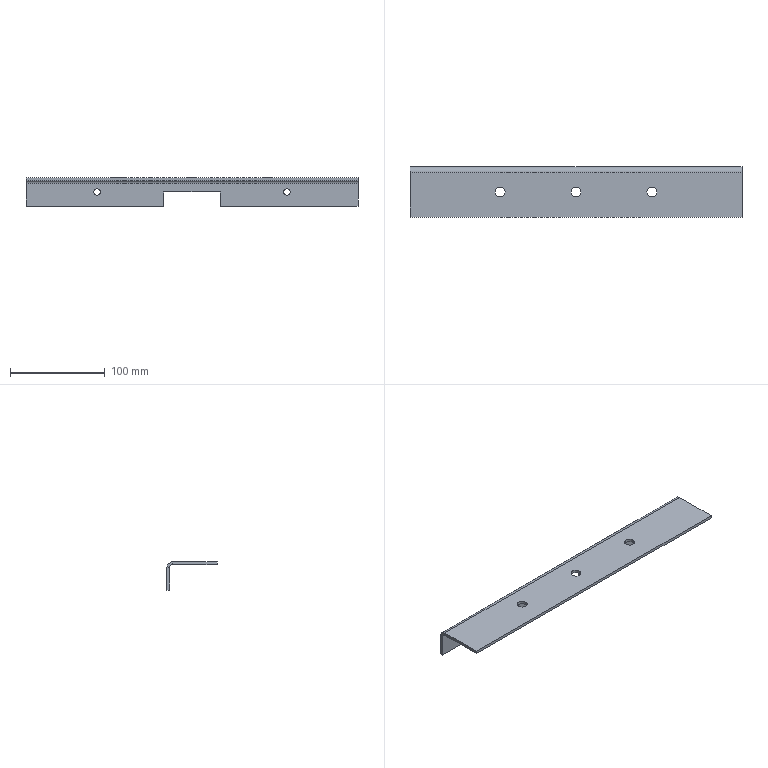Part | SolidWorks | features ICE 3, FlatPattern 1, SMBaseFlange 1, SheetMetal 1 | 1 solid | 28 faces | box 350 x 53 x 30 mm | volume 78262 mm3 | plane 16 | cylinder 12 | commonest cylinder face diameters 10.5 x6 7 x4 6 x1 12 x1
STEP:
#1=CARTESIAN_POINT('',(-100.,-3.,-18.5));
#2=VERTEX_POINT('',#1);
#3=CARTESIAN_POINT('',(-100.,-3.,-11.5));
#4=VERTEX_POINT('',#3);
#5=CARTESIAN_POINT('',(-100.,-3.,-15.));
#6=DIRECTION('',(0.,1.,0.));
#7=DIRECTION('',(0.,0.,-1.));
#8=AXIS2_PLACEMENT_3D('',#5,#6,#7);
#9=CIRCLE('',#8,3.5);
#10=EDGE_CURVE('',#2,#4,#9,.T.);
#11=ORIENTED_EDGE('',*,*,#10,.F.);
#12=CARTESIAN_POINT('',(-100.,0.,-18.5));
#13=VERTEX_POINT('',#12);
#14=CARTESIAN_POINT('',(-100.,-53.001,-18.5));
#15=DIRECTION('',(0.,1.,0.));
#16=VECTOR('',#15,1000.);
#17=LINE('',#14,#16);
#18=EDGE_CURVE('',#2,#13,#17,.T.);
#19=ORIENTED_EDGE('',*,*,#18,.T.);
#20=CARTESIAN_POINT('',(-100.,0.,-11.5));
#21=VERTEX_POINT('',#20);
#22=CARTESIAN_POINT('',(-100.,0.,-15.));
#23=DIRECTION('',(0.,1.,0.));
#24=DIRECTION('',(0.,0.,1.));
#25=AXIS2_PLACEMENT_3D('',#22,#23,#24);
#26=CIRCLE('',#25,3.5);
#27=EDGE_CURVE('',#13,#21,#26,.T.);
#28=ORIENTED_EDGE('',*,*,#27,.T.);
#29=CARTESIAN_POINT('',(-100.,-53.001,-11.5));
#30=DIRECTION('',(0.,1.,0.));
#31=VECTOR('',#30,1000.);
#32=LINE('',#29,#31);
#33=EDGE_CURVE('',#4,#21,#32,.T.);
#34=ORIENTED_EDGE('',*,*,#33,.F.);
#35=EDGE_LOOP('',(#11,#19,#28,#34));
#36=FACE_OUTER_BOUND('',#35,.T.);
#37=CARTESIAN_POINT('',(-100.,-53.001,-15.));
#38=DIRECTION('',(0.,1.,0.));
#39=DIRECTION('',(0.,0.,1.));
#40=AXIS2_PLACEMENT_3D('',#37,#38,#39);
#41=CYLINDRICAL_SURFACE('',#40,3.5);
#42=ADVANCED_FACE('',(#36),#41,.F.);
#43=CARTESIAN_POINT('',(100.,-3.,-18.5));
#44=VERTEX_POINT('',#43);
#45=CARTESIAN_POINT('',(100.,-3.,-11.5));
#46=VERTEX_POINT('',#45);
#47=CARTESIAN_POINT('',(100.,-3.,-15.));
#48=DIRECTION('',(0.,1.,0.));
#49=DIRECTION('',(0.,0.,-1.));
#50=AXIS2_PLACEMENT_3D('',#47,#48,#49);
#51=CIRCLE('',#50,3.5);
#52=EDGE_CURVE('',#44,#46,#51,.T.);
#53=ORIENTED_EDGE('',*,*,#52,.F.);
#54=CARTESIAN_POINT('',(100.,0.,-18.5));
#55=VERTEX_POINT('',#54);
#56=CARTESIAN_POINT('',(100.,-53.001,-18.5));
#57=DIRECTION('',(0.,1.,0.));
#58=VECTOR('',#57,1000.);
#59=LINE('',#56,#58);
#60=EDGE_CURVE('',#44,#55,#59,.T.);
#61=ORIENTED_EDGE('',*,*,#60,.T.);
#62=CARTESIAN_POINT('',(100.,0.,-11.5));
#63=VERTEX_POINT('',#62);
#64=CARTESIAN_POINT('',(100.,0.,-15.));
#65=DIRECTION('',(0.,1.,0.));
#66=DIRECTION('',(0.,0.,-1.));
#67=AXIS2_PLACEMENT_3D('',#64,#65,#66);
#68=CIRCLE('',#67,3.5);
#69=EDGE_CURVE('',#55,#63,#68,.T.);
#70=ORIENTED_EDGE('',*,*,#69,.T.);
#71=CARTESIAN_POINT('',(100.,-53.001,-11.5));
#72=DIRECTION('',(0.,1.,0.));
#73=VECTOR('',#72,1000.);
#74=LINE('',#71,#73);
#75=EDGE_CURVE('',#46,#63,#74,.T.);
#76=ORIENTED_EDGE('',*,*,#75,.F.);
#77=EDGE_LOOP('',(#53,#61,#70,#76));
#78=FACE_OUTER_BOUND('',#77,.T.);
#79=CARTESIAN_POINT('',(100.,-53.001,-15.));
#80=DIRECTION('',(0.,1.,0.));
#81=DIRECTION('',(0.,0.,1.));
#82=AXIS2_PLACEMENT_3D('',#79,#80,#81);
#83=CYLINDRICAL_SURFACE('',#82,3.5);
#84=ADVANCED_FACE('',(#78),#83,.F.);
#85=CARTESIAN_POINT('',(-74.75,-26.5,-3.));
#86=VERTEX_POINT('',#85);
#87=CARTESIAN_POINT('',(-85.25,-26.5,-3.));
#88=VERTEX_POINT('',#87);
#89=CARTESIAN_POINT('',(-80.,-26.5,-3.));
#90=DIRECTION('',(0.,0.,-1.));
#91=DIRECTION('',(-1.,0.,0.));
#92=AXIS2_PLACEMENT_3D('',#89,#90,#91);
#93=CIRCLE('',#92,5.25);
#94=EDGE_CURVE('',#86,#88,#93,.T.);
#95=ORIENTED_EDGE('',*,*,#94,.T.);
#96=CARTESIAN_POINT('',(-85.25,-26.5,0.));
#97=VERTEX_POINT('',#96);
#98=CARTESIAN_POINT('',(-85.25,-26.5,-30.));
#99=DIRECTION('',(0.,0.,1.));
#100=VECTOR('',#99,1000.);
#101=LINE('',#98,#100);
#102=EDGE_CURVE('',#88,#97,#101,.T.);
#103=ORIENTED_EDGE('',*,*,#102,.T.);
#104=CARTESIAN_POINT('',(-74.75,-26.5,0.));
#105=VERTEX_POINT('',#104);
#106=CARTESIAN_POINT('',(-80.,-26.5,0.));
#107=DIRECTION('',(0.,0.,1.));
#108=DIRECTION('',(1.,0.,0.));
#109=AXIS2_PLACEMENT_3D('',#106,#107,#108);
#110=CIRCLE('',#109,5.25);
#111=EDGE_CURVE('',#97,#105,#110,.T.);
#112=ORIENTED_EDGE('',*,*,#111,.T.);
#113=CARTESIAN_POINT('',(-74.75,-26.5,-30.));
#114=DIRECTION('',(0.,0.,1.));
#115=VECTOR('',#114,1000.);
#116=LINE('',#113,#115);
#117=EDGE_CURVE('',#86,#105,#116,.T.);
#118=ORIENTED_EDGE('',*,*,#117,.F.);
#119=EDGE_LOOP('',(#95,#103,#112,#118));
#120=FACE_OUTER_BOUND('',#119,.T.);
#121=CARTESIAN_POINT('',(-80.,-26.5,-30.));
#122=DIRECTION('',(0.,0.,1.));
#123=DIRECTION('',(1.,0.,0.));
#124=AXIS2_PLACEMENT_3D('',#121,#122,#123);
#125=CYLINDRICAL_SURFACE('',#124,5.25);
#126=ADVANCED_FACE('',(#120),#125,.F.);
#127=CARTESIAN_POINT('',(85.25,-26.5,-3.));
#128=VERTEX_POINT('',#127);
#129=CARTESIAN_POINT('',(74.75,-26.5,-3.));
#130=VERTEX_POINT('',#129);
#131=CARTESIAN_POINT('',(80.,-26.5,-3.));
#132=DIRECTION('',(0.,0.,-1.));
#133=DIRECTION('',(-1.,0.,0.));
#134=AXIS2_PLACEMENT_3D('',#131,#132,#133);
#135=CIRCLE('',#134,5.25);
#136=EDGE_CURVE('',#128,#130,#135,.T.);
#137=ORIENTED_EDGE('',*,*,#136,.T.);
#138=CARTESIAN_POINT('',(74.75,-26.5,0.));
#139=VERTEX_POINT('',#138);
#140=CARTESIAN_POINT('',(74.75,-26.5,-30.));
#141=DIRECTION('',(0.,0.,1.));
#142=VECTOR('',#141,1000.);
#143=LINE('',#140,#142);
#144=EDGE_CURVE('',#130,#139,#143,.T.);
#145=ORIENTED_EDGE('',*,*,#144,.T.);
#146=CARTESIAN_POINT('',(85.25,-26.5,0.));
#147=VERTEX_POINT('',#146);
#148=CARTESIAN_POINT('',(80.,-26.5,0.));
#149=DIRECTION('',(0.,0.,1.));
#150=DIRECTION('',(1.,0.,0.));
#151=AXIS2_PLACEMENT_3D('',#148,#149,#150);
#152=CIRCLE('',#151,5.25);
#153=EDGE_CURVE('',#139,#147,#152,.T.);
#154=ORIENTED_EDGE('',*,*,#153,.T.);
#155=CARTESIAN_POINT('',(85.25,-26.5,-30.));
#156=DIRECTION('',(0.,0.,1.));
#157=VECTOR('',#156,1000.);
#158=LINE('',#155,#157);
#159=EDGE_CURVE('',#128,#147,#158,.T.);
#160=ORIENTED_EDGE('',*,*,#159,.F.);
#161=EDGE_LOOP('',(#137,#145,#154,#160));
#162=FACE_OUTER_BOUND('',#161,.T.);
#163=CARTESIAN_POINT('',(80.,-26.5,-30.));
#164=DIRECTION('',(0.,0.,1.));
#165=DIRECTION('',(1.,0.,0.));
#166=AXIS2_PLACEMENT_3D('',#163,#164,#165);
#167=CYLINDRICAL_SURFACE('',#166,5.25);
#168=ADVANCED_FACE('',(#162),#167,.F.);
#169=CARTESIAN_POINT('',(5.25,-26.5,-3.));
#170=VERTEX_POINT('',#169);
#171=CARTESIAN_POINT('',(-5.25,-26.5,-3.));
#172=VERTEX_POINT('',#171);
#173=CARTESIAN_POINT('',(0.,-26.5,-3.));
#174=DIRECTION('',(0.,0.,-1.));
#175=DIRECTION('',(-1.,0.,0.));
#176=AXIS2_PLACEMENT_3D('',#173,#174,#175);
#177=CIRCLE('',#176,5.25);
#178=EDGE_CURVE('',#170,#172,#177,.T.);
#179=ORIENTED_EDGE('',*,*,#178,.T.);
#180=CARTESIAN_POINT('',(-5.25,-26.5,0.));
#181=VERTEX_POINT('',#180);
#182=CARTESIAN_POINT('',(-5.25,-26.5,-30.));
#183=DIRECTION('',(0.,0.,1.));
#184=VECTOR('',#183,1000.);
#185=LINE('',#182,#184);
#186=EDGE_CURVE('',#172,#181,#185,.T.);
#187=ORIENTED_EDGE('',*,*,#186,.T.);
#188=CARTESIAN_POINT('',(5.25,-26.5,0.));
#189=VERTEX_POINT('',#188);
#190=CARTESIAN_POINT('',(0.,-26.5,0.));
#191=DIRECTION('',(0.,0.,1.));
#192=DIRECTION('',(1.,0.,0.));
#193=AXIS2_PLACEMENT_3D('',#190,#191,#192);
#194=CIRCLE('',#193,5.25);
#195=EDGE_CURVE('',#181,#189,#194,.T.);
#196=ORIENTED_EDGE('',*,*,#195,.T.);
#197=CARTESIAN_POINT('',(5.25,-26.5,-30.));
#198=DIRECTION('',(0.,0.,1.));
#199=VECTOR('',#198,1000.);
#200=LINE('',#197,#199);
#201=EDGE_CURVE('',#170,#189,#200,.T.);
#202=ORIENTED_EDGE('',*,*,#201,.F.);
#203=EDGE_LOOP('',(#179,#187,#196,#202));
#204=FACE_OUTER_BOUND('',#203,.T.);
#205=CARTESIAN_POINT('',(0.,-26.5,-30.));
#206=DIRECTION('',(0.,0.,1.));
#207=DIRECTION('',(1.,0.,0.));
#208=AXIS2_PLACEMENT_3D('',#205,#206,#207);
#209=CYLINDRICAL_SURFACE('',#208,5.25);
#210=ADVANCED_FACE('',(#204),#209,.F.);
#211=CARTESIAN_POINT('',(30.,0.,-30.));
#212=VERTEX_POINT('',#211);
#213=CARTESIAN_POINT('',(30.,-3.,-30.));
#214=VERTEX_POINT('',#213);
#215=CARTESIAN_POINT('',(30.,0.,-30.));
#216=DIRECTION('',(0.,-1.,0.));
#217=VECTOR('',#216,1000.);
#218=LINE('',#215,#217);
#219=EDGE_CURVE('',#212,#214,#218,.T.);
#220=ORIENTED_EDGE('',*,*,#219,.F.);
#221=CARTESIAN_POINT('',(175.,0.,-30.));
#222=VERTEX_POINT('',#221);
#223=CARTESIAN_POINT('',(175.,0.,-30.));
#224=DIRECTION('',(-1.,0.,0.));
#225=VECTOR('',#224,1000.);
#226=LINE('',#223,#225);
#227=EDGE_CURVE('',#222,#212,#226,.T.);
#228=ORIENTED_EDGE('',*,*,#227,.F.);
#229=CARTESIAN_POINT('',(175.,-3.,-30.));
#230=VERTEX_POINT('',#229);
#231=CARTESIAN_POINT('',(175.,0.,-30.));
#232=DIRECTION('',(0.,-1.,0.));
#233=VECTOR('',#232,1000.);
#234=LINE('',#231,#233);
#235=EDGE_CURVE('',#222,#230,#234,.T.);
#236=ORIENTED_EDGE('',*,*,#235,.T.);
#237=CARTESIAN_POINT('',(175.,-3.,-30.));
#238=DIRECTION('',(-1.,0.,0.));
#239=VECTOR('',#238,1000.);
#240=LINE('',#237,#239);
#241=EDGE_CURVE('',#230,#214,#240,.T.);
#242=ORIENTED_EDGE('',*,*,#241,.T.);
#243=EDGE_LOOP('',(#220,#228,#236,#242));
#244=FACE_OUTER_BOUND('',#243,.T.);
#245=CARTESIAN_POINT('',(175.,0.,-30.));
#246=DIRECTION('',(0.,0.,-1.));
#247=DIRECTION('',(-1.,0.,0.));
#248=AXIS2_PLACEMENT_3D('',#245,#246,#247);
#249=PLANE('',#248);
#250=ADVANCED_FACE('',(#244),#249,.T.);
#251=CARTESIAN_POINT('',(175.,0.,-6.));
#252=VERTEX_POINT('',#251);
#253=CARTESIAN_POINT('',(175.,-3.,-6.));
#254=VERTEX_POINT('',#253);
#255=CARTESIAN_POINT('',(175.,0.,-6.));
#256=DIRECTION('',(0.,-1.,0.));
#257=VECTOR('',#256,1000.);
#258=LINE('',#255,#257);
#259=EDGE_CURVE('',#252,#254,#258,.T.);
#260=ORIENTED_EDGE('',*,*,#259,.F.);
#261=CARTESIAN_POINT('',(175.,-6.,0.));
#262=VERTEX_POINT('',#261);
#263=CARTESIAN_POINT('',(175.,-6.,-6.));
#264=DIRECTION('',(1.,0.,0.));
#265=DIRECTION('',(0.,0.,1.));
#266=AXIS2_PLACEMENT_3D('',#263,#264,#265);
#267=CIRCLE('',#266,6.);
#268=EDGE_CURVE('',#252,#262,#267,.T.);
#269=ORIENTED_EDGE('',*,*,#268,.T.);
#270=CARTESIAN_POINT('',(175.,-6.,-3.));
#271=VERTEX_POINT('',#270);
#272=CARTESIAN_POINT('',(175.,-6.,-3.));
#273=DIRECTION('',(0.,0.,1.));
#274=VECTOR('',#273,1000.);
#275=LINE('',#272,#274);
#276=EDGE_CURVE('',#271,#262,#275,.T.);
#277=ORIENTED_EDGE('',*,*,#276,.F.);
#278=CARTESIAN_POINT('',(175.,-6.,-6.));
#279=DIRECTION('',(1.,0.,0.));
#280=DIRECTION('',(0.,0.,-1.));
#281=AXIS2_PLACEMENT_3D('',#278,#279,#280);
#282=CIRCLE('',#281,3.);
#283=EDGE_CURVE('',#254,#271,#282,.T.);
#284=ORIENTED_EDGE('',*,*,#283,.F.);
#285=EDGE_LOOP('',(#260,#269,#277,#284));
#286=FACE_OUTER_BOUND('',#285,.T.);
#287=CARTESIAN_POINT('',(175.,0.,-6.));
#288=DIRECTION('',(1.,0.,0.));
#289=DIRECTION('',(0.,0.,-1.));
#290=AXIS2_PLACEMENT_3D('',#287,#288,#289);
#291=PLANE('',#290);
#292=ADVANCED_FACE('',(#286),#291,.T.);
#293=CARTESIAN_POINT('',(175.,0.,-30.));
#294=DIRECTION('',(0.,0.,1.));
#295=VECTOR('',#294,1000.);
#296=LINE('',#293,#295);
#297=EDGE_CURVE('',#222,#252,#296,.T.);
#298=ORIENTED_EDGE('',*,*,#297,.T.);
#299=ORIENTED_EDGE('',*,*,#259,.T.);
#300=CARTESIAN_POINT('',(175.,-3.,-30.));
#301=DIRECTION('',(0.,0.,1.));
#302=VECTOR('',#301,1000.);
#303=LINE('',#300,#302);
#304=EDGE_CURVE('',#230,#254,#303,.T.);
#305=ORIENTED_EDGE('',*,*,#304,.F.);
#306=ORIENTED_EDGE('',*,*,#235,.F.);
#307=EDGE_LOOP('',(#298,#299,#305,#306));
#308=FACE_OUTER_BOUND('',#307,.T.);
#309=CARTESIAN_POINT('',(175.,-6.,-3.));
#310=DIRECTION('',(1.,0.,0.));
#311=DIRECTION('',(0.,0.,-1.));
#312=AXIS2_PLACEMENT_3D('',#309,#310,#311);
#313=PLANE('',#312);
#314=ADVANCED_FACE('',(#308),#313,.T.);
#315=CARTESIAN_POINT('',(-175.,-6.,0.));
#316=VERTEX_POINT('',#315);
#317=CARTESIAN_POINT('',(-175.,-6.,-3.));
#318=VERTEX_POINT('',#317);
#319=CARTESIAN_POINT('',(-175.,-6.,0.));
#320=DIRECTION('',(0.,0.,-1.));
#321=VECTOR('',#320,1000.);
#322=LINE('',#319,#321);
#323=EDGE_CURVE('',#316,#318,#322,.T.);
#324=ORIENTED_EDGE('',*,*,#323,.F.);
#325=CARTESIAN_POINT('',(-175.,0.,-6.));
#326=VERTEX_POINT('',#325);
#327=CARTESIAN_POINT('',(-175.,-6.,-6.));
#328=DIRECTION('',(1.,0.,0.));
#329=DIRECTION('',(0.,0.,1.));
#330=AXIS2_PLACEMENT_3D('',#327,#328,#329);
#331=CIRCLE('',#330,6.);
#332=EDGE_CURVE('',#326,#316,#331,.T.);
#333=ORIENTED_EDGE('',*,*,#332,.F.);
#334=CARTESIAN_POINT('',(-175.,-3.,-6.));
#335=VERTEX_POINT('',#334);
#336=CARTESIAN_POINT('',(-175.,-3.,-6.));
#337=DIRECTION('',(0.,1.,0.));
#338=VECTOR('',#337,1000.);
#339=LINE('',#336,#338);
#340=EDGE_CURVE('',#335,#326,#339,.T.);
#341=ORIENTED_EDGE('',*,*,#340,.F.);
#342=CARTESIAN_POINT('',(-175.,-6.,-6.));
#343=DIRECTION('',(1.,0.,0.));
#344=DIRECTION('',(0.,0.,-1.));
#345=AXIS2_PLACEMENT_3D('',#342,#343,#344);
#346=CIRCLE('',#345,3.);
#347=EDGE_CURVE('',#335,#318,#346,.T.);
#348=ORIENTED_EDGE('',*,*,#347,.T.);
#349=EDGE_LOOP('',(#324,#333,#341,#348));
#350=FACE_OUTER_BOUND('',#349,.T.);
#351=CARTESIAN_POINT('',(-175.,-6.,0.));
#352=DIRECTION('',(-1.,0.,0.));
#353=DIRECTION('',(0.,0.,1.));
#354=AXIS2_PLACEMENT_3D('',#351,#352,#353);
#355=PLANE('',#354);
#356=ADVANCED_FACE('',(#350),#355,.T.);
#357=CARTESIAN_POINT('',(-175.,-53.,0.));
#358=VERTEX_POINT('',#357);
#359=CARTESIAN_POINT('',(-175.,0.,0.));
#360=DIRECTION('',(0.,-1.,0.));
#361=VECTOR('',#360,1000.);
#362=LINE('',#359,#361);
#363=EDGE_CURVE('',#316,#358,#362,.T.);
#364=ORIENTED_EDGE('',*,*,#363,.F.);
#365=ORIENTED_EDGE('',*,*,#323,.T.);
#366=CARTESIAN_POINT('',(-175.,-53.,-3.));
#367=VERTEX_POINT('',#366);
#368=CARTESIAN_POINT('',(-175.,0.,-3.));
#369=DIRECTION('',(0.,-1.,0.));
#370=VECTOR('',#369,1000.);
#371=LINE('',#368,#370);
#372=EDGE_CURVE('',#318,#367,#371,.T.);
#373=ORIENTED_EDGE('',*,*,#372,.T.);
#374=CARTESIAN_POINT('',(-175.,-53.,-3.));
#375=DIRECTION('',(0.,0.,1.));
#376=VECTOR('',#375,1000.);
#377=LINE('',#374,#376);
#378=EDGE_CURVE('',#367,#358,#377,.T.);
#379=ORIENTED_EDGE('',*,*,#378,.T.);
#380=EDGE_LOOP('',(#364,#365,#373,#379));
#381=FACE_OUTER_BOUND('',#380,.T.);
#382=CARTESIAN_POINT('',(-175.,-3.,-6.));
#383=DIRECTION('',(-1.,0.,0.));
#384=DIRECTION('',(0.,0.,1.));
#385=AXIS2_PLACEMENT_3D('',#382,#383,#384);
#386=PLANE('',#385);
#387=ADVANCED_FACE('',(#381),#386,.T.);
#388=CARTESIAN_POINT('',(-80.,-26.5,0.));
#389=DIRECTION('',(0.,0.,1.));
#390=DIRECTION('',(1.,0.,0.));
#391=AXIS2_PLACEMENT_3D('',#388,#389,#390);
#392=CIRCLE('',#391,5.25);
#393=EDGE_CURVE('',#105,#97,#392,.T.);
#394=ORIENTED_EDGE('',*,*,#393,.F.);
#395=ORIENTED_EDGE('',*,*,#111,.F.);
#396=EDGE_LOOP('',(#394,#395));
#397=FACE_BOUND('',#396,.T.);
#398=CARTESIAN_POINT('',(80.,-26.5,0.));
#399=DIRECTION('',(0.,0.,1.));
#400=DIRECTION('',(1.,0.,0.));
#401=AXIS2_PLACEMENT_3D('',#398,#399,#400);
#402=CIRCLE('',#401,5.25);
#403=EDGE_CURVE('',#147,#139,#402,.T.);
#404=ORIENTED_EDGE('',*,*,#403,.F.);
#405=ORIENTED_EDGE('',*,*,#153,.F.);
#406=EDGE_LOOP('',(#404,#405));
#407=FACE_BOUND('',#406,.T.);
#408=CARTESIAN_POINT('',(0.,-26.5,0.));
#409=DIRECTION('',(0.,0.,1.));
#410=DIRECTION('',(1.,0.,0.));
#411=AXIS2_PLACEMENT_3D('',#408,#409,#410);
#412=CIRCLE('',#411,5.25);
#413=EDGE_CURVE('',#189,#181,#412,.T.);
#414=ORIENTED_EDGE('',*,*,#413,.F.);
#415=ORIENTED_EDGE('',*,*,#195,.F.);
#416=EDGE_LOOP('',(#414,#415));
#417=FACE_BOUND('',#416,.T.);
#418=ORIENTED_EDGE('',*,*,#363,.T.);
#419=CARTESIAN_POINT('',(175.,-53.,0.));
#420=VERTEX_POINT('',#419);
#421=CARTESIAN_POINT('',(175.,-53.,0.));
#422=DIRECTION('',(-1.,0.,0.));
#423=VECTOR('',#422,1000.);
#424=LINE('',#421,#423);
#425=EDGE_CURVE('',#420,#358,#424,.T.);
#426=ORIENTED_EDGE('',*,*,#425,.F.);
#427=CARTESIAN_POINT('',(175.,0.,0.));
#428=DIRECTION('',(0.,-1.,0.));
#429=VECTOR('',#428,1000.);
#430=LINE('',#427,#429);
#431=EDGE_CURVE('',#262,#420,#430,.T.);
#432=ORIENTED_EDGE('',*,*,#431,.F.);
#433=CARTESIAN_POINT('',(175.,-6.,0.));
#434=DIRECTION('',(-1.,0.,0.));
#435=VECTOR('',#434,1000.);
#436=LINE('',#433,#435);
#437=EDGE_CURVE('',#262,#316,#436,.T.);
#438=ORIENTED_EDGE('',*,*,#437,.T.);
#439=EDGE_LOOP('',(#418,#426,#432,#438));
#440=FACE_OUTER_BOUND('',#439,.T.);
#441=CARTESIAN_POINT('',(175.,0.,0.));
#442=DIRECTION('',(0.,0.,-1.));
#443=DIRECTION('',(-1.,0.,0.));
#444=AXIS2_PLACEMENT_3D('',#441,#442,#443);
#445=PLANE('',#444);
#446=ADVANCED_FACE('',(#397,#407,#417,#440),#445,.F.);
#447=ORIENTED_EDGE('',*,*,#378,.F.);
#448=CARTESIAN_POINT('',(175.,-53.,-3.));
#449=VERTEX_POINT('',#448);
#450=CARTESIAN_POINT('',(175.,-53.,-3.));
#451=DIRECTION('',(-1.,0.,0.));
#452=VECTOR('',#451,1000.);
#453=LINE('',#450,#452);
#454=EDGE_CURVE('',#449,#367,#453,.T.);
#455=ORIENTED_EDGE('',*,*,#454,.F.);
#456=CARTESIAN_POINT('',(175.,-53.,-3.));
#457=DIRECTION('',(0.,0.,1.));
#458=VECTOR('',#457,1000.);
#459=LINE('',#456,#458);
#460=EDGE_CURVE('',#449,#420,#459,.T.);
#461=ORIENTED_EDGE('',*,*,#460,.T.);
#462=ORIENTED_EDGE('',*,*,#425,.T.);
#463=EDGE_LOOP('',(#447,#455,#461,#462));
#464=FACE_OUTER_BOUND('',#463,.T.);
#465=CARTESIAN_POINT('',(175.,-53.,-3.));
#466=DIRECTION('',(0.,-1.,0.));
#467=DIRECTION('',(0.,0.,-1.));
#468=AXIS2_PLACEMENT_3D('',#465,#466,#467);
#469=PLANE('',#468);
#470=ADVANCED_FACE('',(#464),#469,.T.);
#471=ORIENTED_EDGE('',*,*,#94,.F.);
#472=CARTESIAN_POINT('',(-80.,-26.5,-3.));
#473=DIRECTION('',(0.,0.,-1.));
#474=DIRECTION('',(-1.,0.,0.));
#475=AXIS2_PLACEMENT_3D('',#472,#473,#474);
#476=CIRCLE('',#475,5.25);
#477=EDGE_CURVE('',#88,#86,#476,.T.);
#478=ORIENTED_EDGE('',*,*,#477,.F.);
#479=EDGE_LOOP('',(#471,#478));
#480=FACE_BOUND('',#479,.T.);
#481=ORIENTED_EDGE('',*,*,#136,.F.);
#482=CARTESIAN_POINT('',(80.,-26.5,-3.));
#483=DIRECTION('',(0.,0.,-1.));
#484=DIRECTION('',(-1.,0.,0.));
#485=AXIS2_PLACEMENT_3D('',#482,#483,#484);
#486=CIRCLE('',#485,5.25);
#487=EDGE_CURVE('',#130,#128,#486,.T.);
#488=ORIENTED_EDGE('',*,*,#487,.F.);
#489=EDGE_LOOP('',(#481,#488));
#490=FACE_BOUND('',#489,.T.);
#491=ORIENTED_EDGE('',*,*,#178,.F.);
#492=CARTESIAN_POINT('',(0.,-26.5,-3.));
#493=DIRECTION('',(0.,0.,-1.));
#494=DIRECTION('',(-1.,0.,0.));
#495=AXIS2_PLACEMENT_3D('',#492,#493,#494);
#496=CIRCLE('',#495,5.25);
#497=EDGE_CURVE('',#172,#170,#496,.T.);
#498=ORIENTED_EDGE('',*,*,#497,.F.);
#499=EDGE_LOOP('',(#491,#498));
#500=FACE_BOUND('',#499,.T.);
#501=ORIENTED_EDGE('',*,*,#372,.F.);
#502=CARTESIAN_POINT('',(175.,-6.,-3.));
#503=DIRECTION('',(-1.,0.,0.));
#504=VECTOR('',#503,1000.);
#505=LINE('',#502,#504);
#506=EDGE_CURVE('',#271,#318,#505,.T.);
#507=ORIENTED_EDGE('',*,*,#506,.F.);
#508=CARTESIAN_POINT('',(175.,0.,-3.));
#509=DIRECTION('',(0.,-1.,0.));
#510=VECTOR('',#509,1000.);
#511=LINE('',#508,#510);
#512=EDGE_CURVE('',#271,#449,#511,.T.);
#513=ORIENTED_EDGE('',*,*,#512,.T.);
#514=ORIENTED_EDGE('',*,*,#454,.T.);
#515=EDGE_LOOP('',(#501,#507,#513,#514));
#516=FACE_OUTER_BOUND('',#515,.T.);
#517=CARTESIAN_POINT('',(175.,0.,-3.));
#518=DIRECTION('',(0.,0.,-1.));
#519=DIRECTION('',(-1.,0.,0.));
#520=AXIS2_PLACEMENT_3D('',#517,#518,#519);
#521=PLANE('',#520);
#522=ADVANCED_FACE('',(#480,#490,#500,#516),#521,.T.);
#523=ORIENTED_EDGE('',*,*,#347,.F.);
#524=CARTESIAN_POINT('',(175.,-3.,-6.));
#525=DIRECTION('',(-1.,0.,0.));
#526=VECTOR('',#525,1000.);
#527=LINE('',#524,#526);
#528=EDGE_CURVE('',#254,#335,#527,.T.);
#529=ORIENTED_EDGE('',*,*,#528,.F.);
#530=ORIENTED_EDGE('',*,*,#283,.T.);
#531=ORIENTED_EDGE('',*,*,#506,.T.);
#532=EDGE_LOOP('',(#523,#529,#530,#531));
#533=FACE_OUTER_BOUND('',#532,.T.);
#534=CARTESIAN_POINT('',(175.,-6.,-6.));
#535=DIRECTION('',(-1.,0.,0.));
#536=DIRECTION('',(0.,0.,1.));
#537=AXIS2_PLACEMENT_3D('',#534,#535,#536);
#538=CYLINDRICAL_SURFACE('',#537,3.);
#539=ADVANCED_FACE('',(#533),#538,.F.);
#540=CARTESIAN_POINT('',(30.,-3.,-15.));
#541=VERTEX_POINT('',#540);
#542=CARTESIAN_POINT('',(30.,-3.,-30.));
#543=DIRECTION('',(0.,0.,1.));
#544=VECTOR('',#543,1000.);
#545=LINE('',#542,#544);
#546=EDGE_CURVE('',#214,#541,#545,.T.);
#547=ORIENTED_EDGE('',*,*,#546,.F.);
#548=ORIENTED_EDGE('',*,*,#241,.F.);
#549=ORIENTED_EDGE('',*,*,#304,.T.);
#550=ORIENTED_EDGE('',*,*,#528,.T.);
#551=CARTESIAN_POINT('',(-175.,-3.,-30.));
#552=VERTEX_POINT('',#551);
#553=CARTESIAN_POINT('',(-175.,-3.,-30.));
#554=DIRECTION('',(0.,0.,1.));
#555=VECTOR('',#554,1000.);
#556=LINE('',#553,#555);
#557=EDGE_CURVE('',#552,#335,#556,.T.);
#558=ORIENTED_EDGE('',*,*,#557,.F.);
#559=CARTESIAN_POINT('',(-30.,-3.,-30.));
#560=VERTEX_POINT('',#559);
#561=CARTESIAN_POINT('',(175.,-3.,-30.));
#562=DIRECTION('',(-1.,0.,0.));
#563=VECTOR('',#562,1000.);
#564=LINE('',#561,#563);
#565=EDGE_CURVE('',#560,#552,#564,.T.);
#566=ORIENTED_EDGE('',*,*,#565,.F.);
#567=CARTESIAN_POINT('',(-30.,-3.,-15.));
#568=VERTEX_POINT('',#567);
#569=CARTESIAN_POINT('',(-30.,-3.,-30.));
#570=DIRECTION('',(0.,0.,-1.));
#571=VECTOR('',#570,1000.);
#572=LINE('',#569,#571);
#573=EDGE_CURVE('',#568,#560,#572,.T.);
#574=ORIENTED_EDGE('',*,*,#573,.F.);
#575=CARTESIAN_POINT('',(175.,-3.,-15.));
#576=DIRECTION('',(-1.,0.,0.));
#577=VECTOR('',#576,1000.);
#578=LINE('',#575,#577);
#579=EDGE_CURVE('',#541,#568,#578,.T.);
#580=ORIENTED_EDGE('',*,*,#579,.F.);
#581=EDGE_LOOP('',(#547,#548,#549,#550,#558,#566,#574,#580));
#582=FACE_OUTER_BOUND('',#581,.T.);
#583=CARTESIAN_POINT('',(-100.,-3.,-15.));
#584=DIRECTION('',(0.,1.,0.));
#585=DIRECTION('',(0.,0.,-1.));
#586=AXIS2_PLACEMENT_3D('',#583,#584,#585);
#587=CIRCLE('',#586,3.5);
#588=EDGE_CURVE('',#4,#2,#587,.T.);
#589=ORIENTED_EDGE('',*,*,#588,.T.);
#590=ORIENTED_EDGE('',*,*,#10,.T.);
#591=EDGE_LOOP('',(#589,#590));
#592=FACE_BOUND('',#591,.T.);
#593=CARTESIAN_POINT('',(100.,-3.,-15.));
#594=DIRECTION('',(0.,1.,0.));
#595=DIRECTION('',(0.,0.,-1.));
#596=AXIS2_PLACEMENT_3D('',#593,#594,#595);
#597=CIRCLE('',#596,3.5);
#598=EDGE_CURVE('',#46,#44,#597,.T.);
#599=ORIENTED_EDGE('',*,*,#598,.T.);
#600=ORIENTED_EDGE('',*,*,#52,.T.);
#601=EDGE_LOOP('',(#599,#600));
#602=FACE_BOUND('',#601,.T.);
#603=CARTESIAN_POINT('',(175.,-3.,-30.));
#604=DIRECTION('',(0.,-1.,0.));
#605=DIRECTION('',(0.,0.,-1.));
#606=AXIS2_PLACEMENT_3D('',#603,#604,#605);
#607=PLANE('',#606);
#608=ADVANCED_FACE('',(#582,#592,#602),#607,.T.);
#609=CARTESIAN_POINT('',(-30.,0.,-30.));
#610=VERTEX_POINT('',#609);
#611=CARTESIAN_POINT('',(-30.,0.,-30.));
#612=DIRECTION('',(0.,1.,0.));
#613=VECTOR('',#612,1000.);
#614=LINE('',#611,#613);
#615=EDGE_CURVE('',#560,#610,#614,.T.);
#616=ORIENTED_EDGE('',*,*,#615,.F.);
#617=ORIENTED_EDGE('',*,*,#565,.T.);
#618=CARTESIAN_POINT('',(-175.,0.,-30.));
#619=VERTEX_POINT('',#618);
#620=CARTESIAN_POINT('',(-175.,0.,-30.));
#621=DIRECTION('',(0.,-1.,0.));
#622=VECTOR('',#621,1000.);
#623=LINE('',#620,#622);
#624=EDGE_CURVE('',#619,#552,#623,.T.);
#625=ORIENTED_EDGE('',*,*,#624,.F.);
#626=CARTESIAN_POINT('',(175.,0.,-30.));
#627=DIRECTION('',(-1.,0.,0.));
#628=VECTOR('',#627,1000.);
#629=LINE('',#626,#628);
#630=EDGE_CURVE('',#610,#619,#629,.T.);
#631=ORIENTED_EDGE('',*,*,#630,.F.);
#632=EDGE_LOOP('',(#616,#617,#625,#631));
#633=FACE_OUTER_BOUND('',#632,.T.);
#634=CARTESIAN_POINT('',(175.,0.,-30.));
#635=DIRECTION('',(0.,0.,-1.));
#636=DIRECTION('',(-1.,0.,0.));
#637=AXIS2_PLACEMENT_3D('',#634,#635,#636);
#638=PLANE('',#637);
#639=ADVANCED_FACE('',(#633),#638,.T.);
#640=CARTESIAN_POINT('',(-100.,0.,-15.));
#641=DIRECTION('',(0.,1.,0.));
#642=DIRECTION('',(0.,0.,1.));
#643=AXIS2_PLACEMENT_3D('',#640,#641,#642);
#644=CIRCLE('',#643,3.5);
#645=EDGE_CURVE('',#21,#13,#644,.T.);
#646=ORIENTED_EDGE('',*,*,#645,.F.);
#647=ORIENTED_EDGE('',*,*,#27,.F.);
#648=EDGE_LOOP('',(#646,#647));
#649=FACE_BOUND('',#648,.T.);
#650=CARTESIAN_POINT('',(100.,0.,-15.));
#651=DIRECTION('',(0.,1.,0.));
#652=DIRECTION('',(0.,0.,-1.));
#653=AXIS2_PLACEMENT_3D('',#650,#651,#652);
#654=CIRCLE('',#653,3.5);
#655=EDGE_CURVE('',#63,#55,#654,.T.);
#656=ORIENTED_EDGE('',*,*,#655,.F.);
#657=ORIENTED_EDGE('',*,*,#69,.F.);
#658=EDGE_LOOP('',(#656,#657));
#659=FACE_BOUND('',#658,.T.);
#660=ORIENTED_EDGE('',*,*,#227,.T.);
#661=CARTESIAN_POINT('',(30.,0.,-15.));
#662=VERTEX_POINT('',#661);
#663=CARTESIAN_POINT('',(30.,0.,-15.));
#664=DIRECTION('',(0.,0.,-1.));
#665=VECTOR('',#664,1000.);
#666=LINE('',#663,#665);
#667=EDGE_CURVE('',#662,#212,#666,.T.);
#668=ORIENTED_EDGE('',*,*,#667,.F.);
#669=CARTESIAN_POINT('',(-30.,0.,-15.));
#670=VERTEX_POINT('',#669);
#671=CARTESIAN_POINT('',(-30.,0.,-15.));
#672=DIRECTION('',(1.,0.,0.));
#673=VECTOR('',#672,1000.);
#674=LINE('',#671,#673);
#675=EDGE_CURVE('',#670,#662,#674,.T.);
#676=ORIENTED_EDGE('',*,*,#675,.F.);
#677=CARTESIAN_POINT('',(-30.,0.,-30.));
#678=DIRECTION('',(0.,0.,-1.));
#679=VECTOR('',#678,1000.);
#680=LINE('',#677,#679);
#681=EDGE_CURVE('',#670,#610,#680,.T.);
#682=ORIENTED_EDGE('',*,*,#681,.T.);
#683=ORIENTED_EDGE('',*,*,#630,.T.);
#684=CARTESIAN_POINT('',(-175.,0.,-30.));
#685=DIRECTION('',(0.,0.,1.));
#686=VECTOR('',#685,1000.);
#687=LINE('',#684,#686);
#688=EDGE_CURVE('',#619,#326,#687,.T.);
#689=ORIENTED_EDGE('',*,*,#688,.T.);
#690=CARTESIAN_POINT('',(175.,0.,-6.));
#691=DIRECTION('',(-1.,0.,0.));
#692=VECTOR('',#691,1000.);
#693=LINE('',#690,#692);
#694=EDGE_CURVE('',#252,#326,#693,.T.);
#695=ORIENTED_EDGE('',*,*,#694,.F.);
#696=ORIENTED_EDGE('',*,*,#297,.F.);
#697=EDGE_LOOP('',(#660,#668,#676,#682,#683,#689,#695,#696));
#698=FACE_OUTER_BOUND('',#697,.T.);
#699=CARTESIAN_POINT('',(175.,0.,-30.));
#700=DIRECTION('',(0.,-1.,0.));
#701=DIRECTION('',(0.,0.,-1.));
#702=AXIS2_PLACEMENT_3D('',#699,#700,#701);
#703=PLANE('',#702);
#704=ADVANCED_FACE('',(#649,#659,#698),#703,.F.);
#705=ORIENTED_EDGE('',*,*,#332,.T.);
#706=ORIENTED_EDGE('',*,*,#437,.F.);
#707=ORIENTED_EDGE('',*,*,#268,.F.);
#708=ORIENTED_EDGE('',*,*,#694,.T.);
#709=EDGE_LOOP('',(#705,#706,#707,#708));
#710=FACE_OUTER_BOUND('',#709,.T.);
#711=CARTESIAN_POINT('',(175.,-6.,-6.));
#712=DIRECTION('',(-1.,0.,0.));
#713=DIRECTION('',(0.,0.,1.));
#714=AXIS2_PLACEMENT_3D('',#711,#712,#713);
#715=CYLINDRICAL_SURFACE('',#714,6.);
#716=ADVANCED_FACE('',(#710),#715,.T.);
#717=ORIENTED_EDGE('',*,*,#431,.T.);
#718=ORIENTED_EDGE('',*,*,#460,.F.);
#719=ORIENTED_EDGE('',*,*,#512,.F.);
#720=ORIENTED_EDGE('',*,*,#276,.T.);
#721=EDGE_LOOP('',(#717,#718,#719,#720));
#722=FACE_OUTER_BOUND('',#721,.T.);
#723=CARTESIAN_POINT('',(175.,-6.,-6.));
#724=DIRECTION('',(1.,0.,0.));
#725=DIRECTION('',(0.,0.,-1.));
#726=AXIS2_PLACEMENT_3D('',#723,#724,#725);
#727=PLANE('',#726);
#728=ADVANCED_FACE('',(#722),#727,.T.);
#729=ORIENTED_EDGE('',*,*,#557,.T.);
#730=ORIENTED_EDGE('',*,*,#340,.T.);
#731=ORIENTED_EDGE('',*,*,#688,.F.);
#732=ORIENTED_EDGE('',*,*,#624,.T.);
#733=EDGE_LOOP('',(#729,#730,#731,#732));
#734=FACE_OUTER_BOUND('',#733,.T.);
#735=CARTESIAN_POINT('',(-175.,-6.,-6.));
#736=DIRECTION('',(1.,0.,0.));
#737=DIRECTION('',(0.,0.,-1.));
#738=AXIS2_PLACEMENT_3D('',#735,#736,#737);
#739=PLANE('',#738);
#740=ADVANCED_FACE('',(#734),#739,.F.);
#741=ORIENTED_EDGE('',*,*,#186,.F.);
#742=ORIENTED_EDGE('',*,*,#497,.T.);
#743=ORIENTED_EDGE('',*,*,#201,.T.);
#744=ORIENTED_EDGE('',*,*,#413,.T.);
#745=EDGE_LOOP('',(#741,#742,#743,#744));
#746=FACE_OUTER_BOUND('',#745,.T.);
#747=CARTESIAN_POINT('',(0.,-26.5,-30.));
#748=DIRECTION('',(0.,0.,1.));
#749=DIRECTION('',(1.,0.,0.));
#750=AXIS2_PLACEMENT_3D('',#747,#748,#749);
#751=CYLINDRICAL_SURFACE('',#750,5.25);
#752=ADVANCED_FACE('',(#746),#751,.F.);
#753=ORIENTED_EDGE('',*,*,#144,.F.);
#754=ORIENTED_EDGE('',*,*,#487,.T.);
#755=ORIENTED_EDGE('',*,*,#159,.T.);
#756=ORIENTED_EDGE('',*,*,#403,.T.);
#757=EDGE_LOOP('',(#753,#754,#755,#756));
#758=FACE_OUTER_BOUND('',#757,.T.);
#759=CARTESIAN_POINT('',(80.,-26.5,-30.));
#760=DIRECTION('',(0.,0.,1.));
#761=DIRECTION('',(1.,0.,0.));
#762=AXIS2_PLACEMENT_3D('',#759,#760,#761);
#763=CYLINDRICAL_SURFACE('',#762,5.25);
#764=ADVANCED_FACE('',(#758),#763,.F.);
#765=ORIENTED_EDGE('',*,*,#102,.F.);
#766=ORIENTED_EDGE('',*,*,#477,.T.);
#767=ORIENTED_EDGE('',*,*,#117,.T.);
#768=ORIENTED_EDGE('',*,*,#393,.T.);
#769=EDGE_LOOP('',(#765,#766,#767,#768));
#770=FACE_OUTER_BOUND('',#769,.T.);
#771=CARTESIAN_POINT('',(-80.,-26.5,-30.));
#772=DIRECTION('',(0.,0.,1.));
#773=DIRECTION('',(1.,0.,0.));
#774=AXIS2_PLACEMENT_3D('',#771,#772,#773);
#775=CYLINDRICAL_SURFACE('',#774,5.25);
#776=ADVANCED_FACE('',(#770),#775,.F.);
#777=ORIENTED_EDGE('',*,*,#60,.F.);
#778=ORIENTED_EDGE('',*,*,#598,.F.);
#779=ORIENTED_EDGE('',*,*,#75,.T.);
#780=ORIENTED_EDGE('',*,*,#655,.T.);
#781=EDGE_LOOP('',(#777,#778,#779,#780));
#782=FACE_OUTER_BOUND('',#781,.T.);
#783=CARTESIAN_POINT('',(100.,-53.001,-15.));
#784=DIRECTION('',(0.,1.,0.));
#785=DIRECTION('',(0.,0.,1.));
#786=AXIS2_PLACEMENT_3D('',#783,#784,#785);
#787=CYLINDRICAL_SURFACE('',#786,3.5);
#788=ADVANCED_FACE('',(#782),#787,.F.);
#789=ORIENTED_EDGE('',*,*,#18,.F.);
#790=ORIENTED_EDGE('',*,*,#588,.F.);
#791=ORIENTED_EDGE('',*,*,#33,.T.);
#792=ORIENTED_EDGE('',*,*,#645,.T.);
#793=EDGE_LOOP('',(#789,#790,#791,#792));
#794=FACE_OUTER_BOUND('',#793,.T.);
#795=CARTESIAN_POINT('',(-100.,-53.001,-15.));
#796=DIRECTION('',(0.,1.,0.));
#797=DIRECTION('',(0.,0.,1.));
#798=AXIS2_PLACEMENT_3D('',#795,#796,#797);
#799=CYLINDRICAL_SURFACE('',#798,3.5);
#800=ADVANCED_FACE('',(#794),#799,.F.);
#801=ORIENTED_EDGE('',*,*,#546,.T.);
#802=CARTESIAN_POINT('',(30.,-53.,-15.));
#803=DIRECTION('',(0.,1.,0.));
#804=VECTOR('',#803,1000.);
#805=LINE('',#802,#804);
#806=EDGE_CURVE('',#541,#662,#805,.T.);
#807=ORIENTED_EDGE('',*,*,#806,.T.);
#808=ORIENTED_EDGE('',*,*,#667,.T.);
#809=ORIENTED_EDGE('',*,*,#219,.T.);
#810=EDGE_LOOP('',(#801,#807,#808,#809));
#811=FACE_OUTER_BOUND('',#810,.T.);
#812=CARTESIAN_POINT('',(30.,-53.,-15.));
#813=DIRECTION('',(1.,0.,0.));
#814=DIRECTION('',(0.,0.,-1.));
#815=AXIS2_PLACEMENT_3D('',#812,#813,#814);
#816=PLANE('',#815);
#817=ADVANCED_FACE('',(#811),#816,.F.);
#818=ORIENTED_EDGE('',*,*,#579,.T.);
#819=CARTESIAN_POINT('',(-30.,-53.,-15.));
#820=DIRECTION('',(0.,1.,0.));
#821=VECTOR('',#820,1000.);
#822=LINE('',#819,#821);
#823=EDGE_CURVE('',#568,#670,#822,.T.);
#824=ORIENTED_EDGE('',*,*,#823,.T.);
#825=ORIENTED_EDGE('',*,*,#675,.T.);
#826=ORIENTED_EDGE('',*,*,#806,.F.);
#827=EDGE_LOOP('',(#818,#824,#825,#826));
#828=FACE_OUTER_BOUND('',#827,.T.);
#829=CARTESIAN_POINT('',(-30.,-53.,-15.));
#830=DIRECTION('',(0.,0.,1.));
#831=DIRECTION('',(1.,0.,0.));
#832=AXIS2_PLACEMENT_3D('',#829,#830,#831);
#833=PLANE('',#832);
#834=ADVANCED_FACE('',(#828),#833,.F.);
#835=ORIENTED_EDGE('',*,*,#573,.T.);
#836=ORIENTED_EDGE('',*,*,#615,.T.);
#837=ORIENTED_EDGE('',*,*,#681,.F.);
#838=ORIENTED_EDGE('',*,*,#823,.F.);
#839=EDGE_LOOP('',(#835,#836,#837,#838));
#840=FACE_OUTER_BOUND('',#839,.T.);
#841=CARTESIAN_POINT('',(-30.,-53.,-15.));
#842=DIRECTION('',(-1.,0.,0.));
#843=DIRECTION('',(0.,0.,1.));
#844=AXIS2_PLACEMENT_3D('',#841,#842,#843);
#845=PLANE('',#844);
#846=ADVANCED_FACE('',(#840),#845,.F.);
#847=CLOSED_SHELL('',(#42,#84,#126,#168,#210,#250,#292,#314,#356,#387,#446,#470,#522,#539,#608,#639,#704,#716,#728,#740,#752,#764,#776,#788,#800,#817,#834,#846));
#848=MANIFOLD_SOLID_BREP('',#847);
#849=CARTESIAN_POINT('',(0.,0.,0.));
#850=DIRECTION('',(0.,0.,1.));
#851=DIRECTION('',(1.,0.,0.));
#852=AXIS2_PLACEMENT_3D('',#849,#850,#851);
#853=(LENGTH_UNIT()NAMED_UNIT(*)SI_UNIT(.MILLI.,.METRE.));
#854=UNCERTAINTY_MEASURE_WITH_UNIT(LENGTH_MEASURE(0.00001),#853,'','');
#855=(NAMED_UNIT(*)PLANE_ANGLE_UNIT()SI_UNIT($,.RADIAN.));
#856=(NAMED_UNIT(*)SI_UNIT($,.STERADIAN.)SOLID_ANGLE_UNIT());
#857=(GEOMETRIC_REPRESENTATION_CONTEXT(3)GLOBAL_UNCERTAINTY_ASSIGNED_CONTEXT((#854))GLOBAL_UNIT_ASSIGNED_CONTEXT((#853,#855,#856))REPRESENTATION_CONTEXT('',''));
#858=ADVANCED_BREP_SHAPE_REPRESENTATION('',(#848,#852),#857);